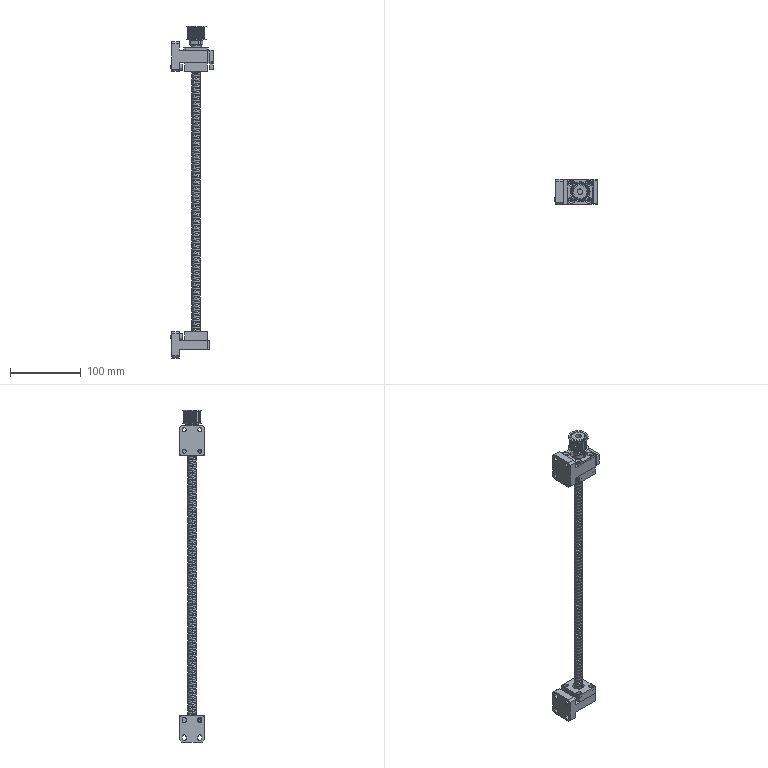Part | NX | features BREP 13 | 15 solids | 994 faces | box 60.5 x 35 x 468 mm | volume 138919 mm3 | cylinder 524 | plane 220 | cone 87 | torus 82 | sphere 78 | spline 3 | commonest cylinder face diameters 12 x153 0.34 x69 2.06 x40 10 x30 3.3 x26 24.07 x26